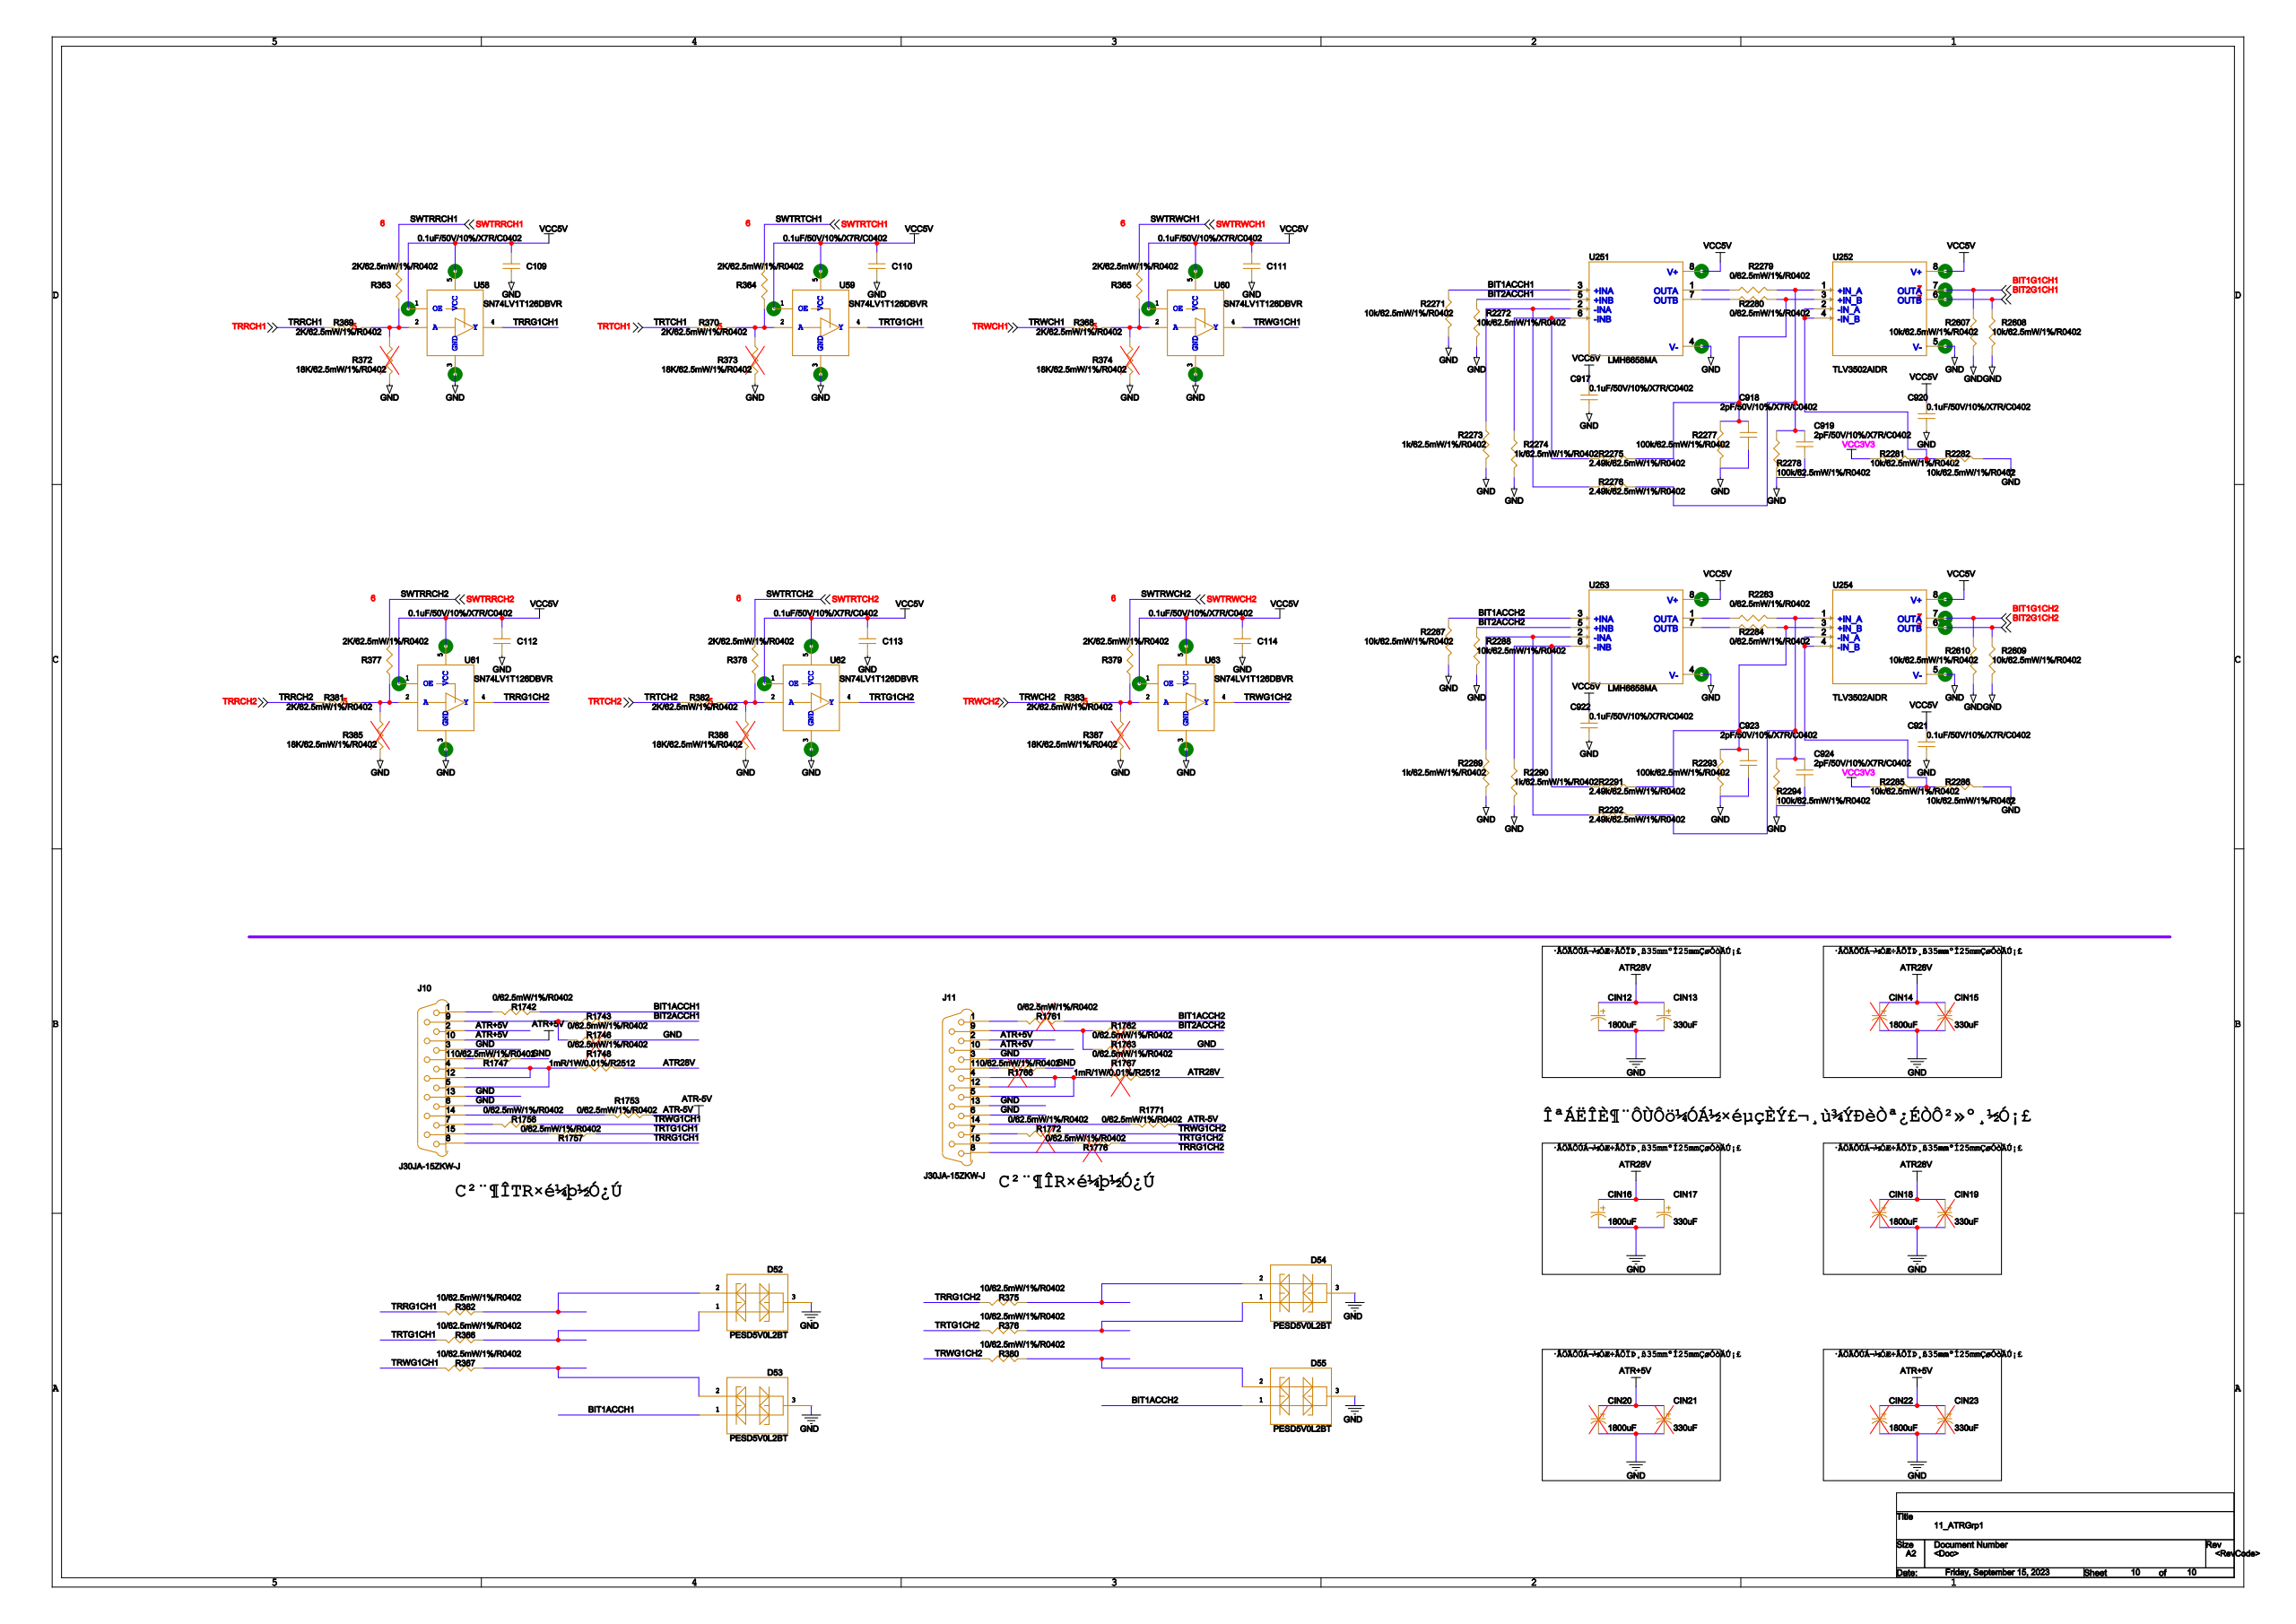Circuit board | Cadence Allegro | 634 parts | 645 nets | one sheet of the schematic
Parts on this sheet (reference | value | footprint):
C109 | 0.1uF/50V/10%/X7R/C0402 | 0402
C110 | 0.1uF/50V/10%/X7R/C0402 | 0402
C111 | 0.1uF/50V/10%/X7R/C0402 | 0402
C112 | 0.1uF/50V/10%/X7R/C0402 | 0402
C113 | 0.1uF/50V/10%/X7R/C0402 | 0402
C114 | 0.1uF/50V/10%/X7R/C0402 | 0402
C918 | 2pF/50V/10%/X7R/C0402 | 0402
C919 | 2pF/50V/10%/X7R/C0402 | 0402
C920 | 0.1uF/50V/10%/X7R/C0402 | 0402
C921 | 0.1uF/50V/10%/X7R/C0402 | 0402
C923 | 2pF/50V/10%/X7R/C0402 | 0402
C924 | 2pF/50V/10%/X7R/C0402 | 0402
CIN12 | ECF1HM182M27OTPO | AP-SMD_BD18-L27-W6_6-LS7_21
CIN13 | ECF1JM331G20OTPO | AP-SMD_BD10-L20-W6_6-LS7_21
CIN14 | ECF1HM182M27OTPO | AP-SMD_BD18-L27-W6_6-LS7_21
CIN15 | ECF1JM331G20OTPO | AP-SMD_BD10-L20-W6_6-LS7_21
CIN16 | ECF1HM182M27OTPO | AP-SMD_BD18-L27-W6_6-LS7_21
CIN17 | ECF1JM331G20OTPO | AP-SMD_BD10-L20-W6_6-LS7_21
CIN18 | ECF1HM182M27OTPO | AP-SMD_BD18-L27-W6_6-LS7_21
CIN19 | ECF1JM331G20OTPO | AP-SMD_BD10-L20-W6_6-LS7_21
CIN20 | ECF1HM182M27OTPO | AP-SMD_BD18-L27-W6_6-LS7_21
CIN21 | ECF1JM331G20OTPO | AP-SMD_BD10-L20-W6_6-LS7_21
CIN22 | ECF1HM182M27OTPO | AP-SMD_BD18-L27-W6_6-LS7_21
CIN23 | ECF1JM331G20OTPO | AP-SMD_BD10-L20-W6_6-LS7_21
D52 | PESD5V0L2BT | SOT23
D53 | PESD5V0L2BT | SOT23
D54 | PESD5V0L2BT | SOT23
D55 | PESD5V0L2BT | SOT23
J10 | J30JA-15ZKW-J | J30JA-15ZKW-J
J11 | J30JA-15ZKW-J | J30JA-15ZKW-J
R362 | 10/62.5mW/1%/R0402 | 0402
R363 | 2K/62.5mW/1%/R0402 | 0402
R364 | 2K/62.5mW/1%/R0402 | 0402
R365 | 2K/62.5mW/1%/R0402 | 0402
R366 | 10/62.5mW/1%/R0402 | 0402
R367 | 10/62.5mW/1%/R0402 | 0402
R368 | 2K/62.5mW/1%/R0402 | 0402
R369 | 2K/62.5mW/1%/R0402 | 0402
R370 | 2K/62.5mW/1%/R0402 | 0402
R372 | 18K/62.5mW/1%/R0402 | 0402
R373 | 18K/62.5mW/1%/R0402 | 0402
R374 | 18K/62.5mW/1%/R0402 | 0402
R375 | 10/62.5mW/1%/R0402 | 0402
R376 | 10/62.5mW/1%/R0402 | 0402
R377 | 2K/62.5mW/1%/R0402 | 0402
R378 | 2K/62.5mW/1%/R0402 | 0402
R379 | 2K/62.5mW/1%/R0402 | 0402
R380 | 10/62.5mW/1%/R0402 | 0402
R381 | 2K/62.5mW/1%/R0402 | 0402
R382 | 2K/62.5mW/1%/R0402 | 0402
R383 | 2K/62.5mW/1%/R0402 | 0402
R385 | 18K/62.5mW/1%/R0402 | 0402
R386 | 18K/62.5mW/1%/R0402 | 0402
R387 | 18K/62.5mW/1%/R0402 | 0402
R1742 | 0/62.5mW/1%/R0402 | 0402
R1743 | 0/62.5mW/1%/R0402 | 0402
R1746 | 0/62.5mW/1%/R0402 | 0402
R1747 | 0/62.5mW/1%/R0402 | 0402
R1748 | 1mR/1W/0.01%/R2512 | 2512
R1753 | 0/62.5mW/1%/R0402 | 0402
R1756 | 0/62.5mW/1%/R0402 | 0402
R1757 | 0/62.5mW/1%/R0402 | 0402
R1761 | 0/62.5mW/1%/R0402 | 0402
R1762 | 0/62.5mW/1%/R0402 | 0402
R1763 | 0/62.5mW/1%/R0402 | 0402
R1766 | 0/62.5mW/1%/R0402 | 0402
R1767 | 1mR/1W/0.01%/R2512 | 2512
R1771 | 0/62.5mW/1%/R0402 | 0402
R1772 | 0/62.5mW/1%/R0402 | 0402
R1776 | 0/62.5mW/1%/R0402 | 0402
R2271 | 10k/62.5mW/1%/R0402 | 0402
R2272 | 10k/62.5mW/1%/R0402 | 0402
R2273 | 1K/62.5mW/1%/R0402 | 0402
R2274 | 1K/62.5mW/1%/R0402 | 0402
R2276 | 2.49k/62.5mW/1%/R0402 | 0402
R2277 | 100k/62.5mW/1%/R0402 | 0402
R2278 | 100k/62.5mW/1%/R0402 | 0402
R2279 | 0/62.5mW/1%/R0402 | 0402
R2280 | 0/62.5mW/1%/R0402 | 0402
R2281 | 10k/62.5mW/1%/R0402 | 0402
R2282 | 10k/62.5mW/1%/R0402 | 0402
R2283 | 0/62.5mW/1%/R0402 | 0402
R2284 | 0/62.5mW/1%/R0402 | 0402
R2285 | 10k/62.5mW/1%/R0402 | 0402
R2286 | 10k/62.5mW/1%/R0402 | 0402
R2287 | 10k/62.5mW/1%/R0402 | 0402
R2288 | 10k/62.5mW/1%/R0402 | 0402
R2289 | 1K/62.5mW/1%/R0402 | 0402
R2290 | 1K/62.5mW/1%/R0402 | 0402
R2292 | 2.49k/62.5mW/1%/R0402 | 0402
R2293 | 100k/62.5mW/1%/R0402 | 0402
R2294 | 100k/62.5mW/1%/R0402 | 0402
R2607 | 10k/62.5mW/1%/R0402 | 0402
R2608 | 10k/62.5mW/1%/R0402 | 0402
R2609 | 10k/62.5mW/1%/R0402 | 0402
R2610 | 10k/62.5mW/1%/R0402 | 0402
U58 | SN74LV1T126DBVR | SOT-23-5
U59 | SN74LV1T126DBVR | SOT-23-5
U60 | SN74LV1T126DBVR | SOT-23-5
U61 | SN74LV1T126DBVR | SOT-23-5
U62 | SN74LV1T126DBVR | SOT-23-5
U63 | SN74LV1T126DBVR | SOT-23-5
U251 | LMH6658MA | SOIC127P599X175-8N
U254 | TLV3502AIDR | SOIC127P599X175-8N
Nets of these parts (net: part-pin ...):
N24662800: J10-1 R1742-2
ATR+5V: CIN20-1 CIN21-1 CIN22-1 CIN23-1 J10-2 J10-10 J11-2 J11-10
N24662819: J10-11 R1747-2
N24662821: J10-4 J10-5 J10-12 R1748-1
AGND: C109-2 C110-2 C111-2 C112-2 C113-2 C114-2 C918-2 C919-2 C920-2 C921-2 C923-2 C924-2 CIN12-2 CIN13-2 CIN14-2 CIN15-2 CIN16-2 CIN17-2 CIN18-2 CIN19-2 CIN20-2 CIN21-2 CIN22-2 CIN23-2 D52-3 D53-3 D54-3 D55-3 J10-3 J10-6 J10-13 J11-3 J11-6 J11-13 R372-1 R373-1 R374-1 R385-1 R386-1 R387-1 R1746-1 R1747-1 R1763-1 R1766-1 R2271-2 R2272-2 R2273-2 R2274-2 R2277-2 R2278-2 R2282-2 R2286-2 R2287-2 R2288-2 R2289-2 R2290-2 R2293-2 R2294-2 R2607-2 R2608-2 R2609-2 R2610-2 U58-3 U59-3 U60-3 U61-3 U62-3 U63-3 U251-4 U254-5
N24662833: J10-14 R1753-2
N24662837: J10-15 R1757-2
N24662835: J10-7 R1756-2
TRRG1CH1: J10-8 R362-2 U58-4
N24662802: J10-9 R1743-2 R1746-2
N24662947: J11-1 R1761-2
N24662960: J11-11 R1766-2
N24662965: J11-4 J11-5 J11-12 R1767-1
N24662977: J11-14 R1771-2
N24662981: J11-15 R1776-2
N24662979: J11-7 R1772-2
TRRG1CH2: J11-8 R375-2 U61-4
N24662949: J11-9 R1762-2 R1763-2
ATR28V: CIN12-1 CIN13-1 CIN14-1 CIN15-1 CIN16-1 CIN17-1 CIN18-1 CIN19-1 R1748-2 R1767-2
ATR-5V: R1753-1 R1771-1
3.3V: R2281-1 R2285-1
VCC5V: C109-1 C110-1 C111-1 C112-1 C113-1 C114-1 C920-1 C921-1 U58-1 U58-5 U59-1 U59-5 U60-1 U60-5 U61-1 U61-5 U62-1 U62-5 U63-1 U63-5 U251-8 U254-8
N24663207: C918-1 R2277-1 R2280-2
N24663205: C919-1 R2276-2 R2278-1 R2279-2
N24662064: C923-1 R2284-2 R2293-1 U254-3
N24662062: C924-1 R2283-2 R2292-2 R2294-1 U254-1
N24663197: R2274-1 U251-6
N24663193: R2273-1 R2276-1 U251-2
N24662046: R2290-1
N24662034: R2289-1 R2292-1
N24663094: D52-2 R362-1
N24661531: D52-1 R366-1
TRTG1CH1: R366-2 R1757-1 U59-4
N24661537: D53-2 R367-1
TRWG1CH1: R367-2 R1756-1 U60-4
N24663963: D54-2 R375-1
N24663940: D54-1 R376-1
TRTG1CH2: R376-2 R1776-1 U62-4
N24663946: D55-2 R380-1
TRWG1CH2: R380-2 R1772-1 U63-4
N24663312: R363-2 R369-2 R372-2 U58-2
N24661559: R364-2 R370-2 R373-2 U59-2
N24662541: R365-2 R368-2 R374-2 U60-2
N24662419: R377-2 R381-2 R385-2 U61-2
N24661572: R378-2 R382-2 R386-2 U62-2
N24661799: R379-2 R383-2 R387-2 U63-2
BIT1ACCH1: D53-1 R1742-1 R2271-1 U251-3
BIT2ACCH1: R1743-1 R2272-1 U251-5
N24663201: R2279-1 U251-1
N24663203: R2280-1 U251-7
BIT1ACCH2: D55-1 R1761-1 R2287-1
BIT2ACCH2: R1762-1 R2288-1
N24662050: R2283-1
N24662052: R2284-1
N24663257: R2281-2 R2282-1
BIT1G1CH1: R2607-1
BIT2G1CH1: R2608-1
N24662114: R2285-2 R2286-1 U254-2 U254-4
BIT1G1CH2: R2610-1 U254-7
BIT2G1CH2: R2609-1 U254-6
SWTRRCH1: R363-1
SWTRTCH1: R364-1
SWTRWCH1: R365-1
TRWCH1: R368-1
TRRCH1: R369-1
TRTCH1: R370-1
SWTRRCH2: R377-1
SWTRTCH2: R378-1
SWTRWCH2: R379-1
TRRCH2: R381-1
TRTCH2: R382-1
TRWCH2: R383-1